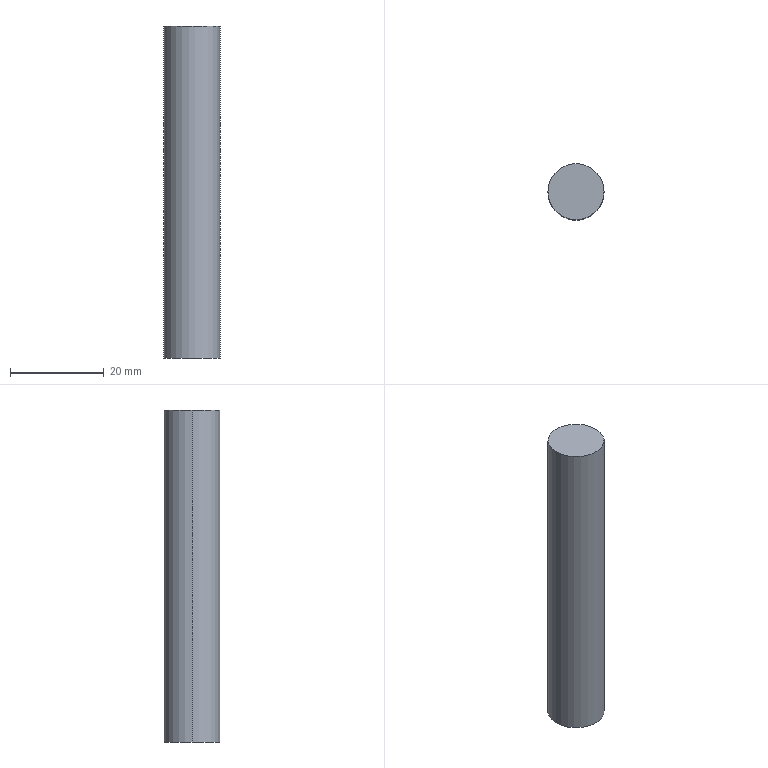Part | SolidWorks | features Extrusion 1 | 1 solid | 4 faces | box 12 x 12 x 71 mm | volume 8030 mm3 | cylinder 2 | plane 2 | commonest cylinder face diameters 12 x2
STEP:
#1=CARTESIAN_POINT('',(6.,0.,35.5));
#2=VERTEX_POINT('',#1);
#3=CARTESIAN_POINT('',(-6.,0.,35.5));
#4=VERTEX_POINT('',#3);
#5=CARTESIAN_POINT('',(0.,0.,35.5));
#6=DIRECTION('',(0.,0.,1.));
#7=DIRECTION('',(1.,0.,0.));
#8=AXIS2_PLACEMENT_3D('',#5,#6,#7);
#9=CIRCLE('',#8,6.);
#10=EDGE_CURVE('',#2,#4,#9,.T.);
#11=ORIENTED_EDGE('',*,*,#10,.F.);
#12=CARTESIAN_POINT('',(6.,0.,-35.5));
#13=VERTEX_POINT('',#12);
#14=CARTESIAN_POINT('',(6.,0.,35.5));
#15=DIRECTION('',(0.,0.,-1.));
#16=VECTOR('',#15,1000.);
#17=LINE('',#14,#16);
#18=EDGE_CURVE('',#2,#13,#17,.T.);
#19=ORIENTED_EDGE('',*,*,#18,.T.);
#20=CARTESIAN_POINT('',(-6.,0.,-35.5));
#21=VERTEX_POINT('',#20);
#22=CARTESIAN_POINT('',(0.,0.,-35.5));
#23=DIRECTION('',(0.,0.,1.));
#24=DIRECTION('',(1.,0.,0.));
#25=AXIS2_PLACEMENT_3D('',#22,#23,#24);
#26=CIRCLE('',#25,6.);
#27=EDGE_CURVE('',#13,#21,#26,.T.);
#28=ORIENTED_EDGE('',*,*,#27,.T.);
#29=CARTESIAN_POINT('',(-6.,0.,35.5));
#30=DIRECTION('',(0.,0.,-1.));
#31=VECTOR('',#30,1000.);
#32=LINE('',#29,#31);
#33=EDGE_CURVE('',#4,#21,#32,.T.);
#34=ORIENTED_EDGE('',*,*,#33,.F.);
#35=EDGE_LOOP('',(#11,#19,#28,#34));
#36=FACE_OUTER_BOUND('',#35,.T.);
#37=CARTESIAN_POINT('',(0.,0.,35.5));
#38=DIRECTION('',(0.,0.,-1.));
#39=DIRECTION('',(-1.,0.,0.));
#40=AXIS2_PLACEMENT_3D('',#37,#38,#39);
#41=CYLINDRICAL_SURFACE('',#40,6.);
#42=ADVANCED_FACE('',(#36),#41,.T.);
#43=ORIENTED_EDGE('',*,*,#18,.F.);
#44=CARTESIAN_POINT('',(0.,0.,35.5));
#45=DIRECTION('',(0.,0.,1.));
#46=DIRECTION('',(1.,0.,0.));
#47=AXIS2_PLACEMENT_3D('',#44,#45,#46);
#48=CIRCLE('',#47,6.);
#49=EDGE_CURVE('',#4,#2,#48,.T.);
#50=ORIENTED_EDGE('',*,*,#49,.F.);
#51=ORIENTED_EDGE('',*,*,#33,.T.);
#52=CARTESIAN_POINT('',(0.,0.,-35.5));
#53=DIRECTION('',(0.,0.,1.));
#54=DIRECTION('',(1.,0.,0.));
#55=AXIS2_PLACEMENT_3D('',#52,#53,#54);
#56=CIRCLE('',#55,6.);
#57=EDGE_CURVE('',#21,#13,#56,.T.);
#58=ORIENTED_EDGE('',*,*,#57,.T.);
#59=EDGE_LOOP('',(#43,#50,#51,#58));
#60=FACE_OUTER_BOUND('',#59,.T.);
#61=CARTESIAN_POINT('',(0.,0.,35.5));
#62=DIRECTION('',(0.,0.,-1.));
#63=DIRECTION('',(-1.,0.,0.));
#64=AXIS2_PLACEMENT_3D('',#61,#62,#63);
#65=CYLINDRICAL_SURFACE('',#64,6.);
#66=ADVANCED_FACE('',(#60),#65,.T.);
#67=ORIENTED_EDGE('',*,*,#49,.T.);
#68=ORIENTED_EDGE('',*,*,#10,.T.);
#69=EDGE_LOOP('',(#67,#68));
#70=FACE_OUTER_BOUND('',#69,.T.);
#71=CARTESIAN_POINT('',(0.,0.,35.5));
#72=DIRECTION('',(0.,0.,1.));
#73=DIRECTION('',(1.,0.,0.));
#74=AXIS2_PLACEMENT_3D('',#71,#72,#73);
#75=PLANE('',#74);
#76=ADVANCED_FACE('',(#70),#75,.T.);
#77=ORIENTED_EDGE('',*,*,#57,.F.);
#78=ORIENTED_EDGE('',*,*,#27,.F.);
#79=EDGE_LOOP('',(#77,#78));
#80=FACE_OUTER_BOUND('',#79,.T.);
#81=CARTESIAN_POINT('',(0.,0.,-35.5));
#82=DIRECTION('',(0.,0.,1.));
#83=DIRECTION('',(1.,0.,0.));
#84=AXIS2_PLACEMENT_3D('',#81,#82,#83);
#85=PLANE('',#84);
#86=ADVANCED_FACE('',(#80),#85,.F.);
#87=CLOSED_SHELL('',(#42,#66,#76,#86));
#88=MANIFOLD_SOLID_BREP('',#87);
#89=CARTESIAN_POINT('',(0.,0.,0.));
#90=DIRECTION('',(0.,0.,1.));
#91=DIRECTION('',(1.,0.,0.));
#92=AXIS2_PLACEMENT_3D('',#89,#90,#91);
#93=(LENGTH_UNIT()NAMED_UNIT(*)SI_UNIT(.MILLI.,.METRE.));
#94=UNCERTAINTY_MEASURE_WITH_UNIT(LENGTH_MEASURE(0.00001),#93,'','');
#95=(NAMED_UNIT(*)PLANE_ANGLE_UNIT()SI_UNIT($,.RADIAN.));
#96=(NAMED_UNIT(*)SI_UNIT($,.STERADIAN.)SOLID_ANGLE_UNIT());
#97=(GEOMETRIC_REPRESENTATION_CONTEXT(3)GLOBAL_UNCERTAINTY_ASSIGNED_CONTEXT((#94))GLOBAL_UNIT_ASSIGNED_CONTEXT((#93,#95,#96))REPRESENTATION_CONTEXT('',''));
#98=ADVANCED_BREP_SHAPE_REPRESENTATION('',(#88,#92),#97);